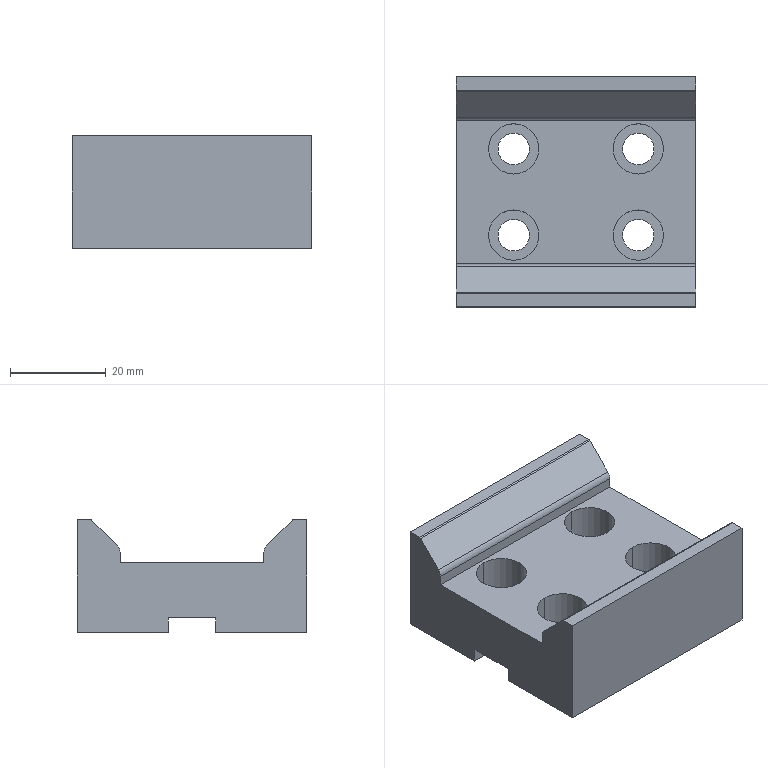Part | STEP file | J454-EBZ05-35-04-Part-1-4 | 1 solid | 40 faces | box 50 x 48 x 23.5 mm | volume 35481 mm3 | cylinder 20 | plane 20 | commonest cylinder face diameters 6.6 x8 10.5 x8 1 x2 4 x2